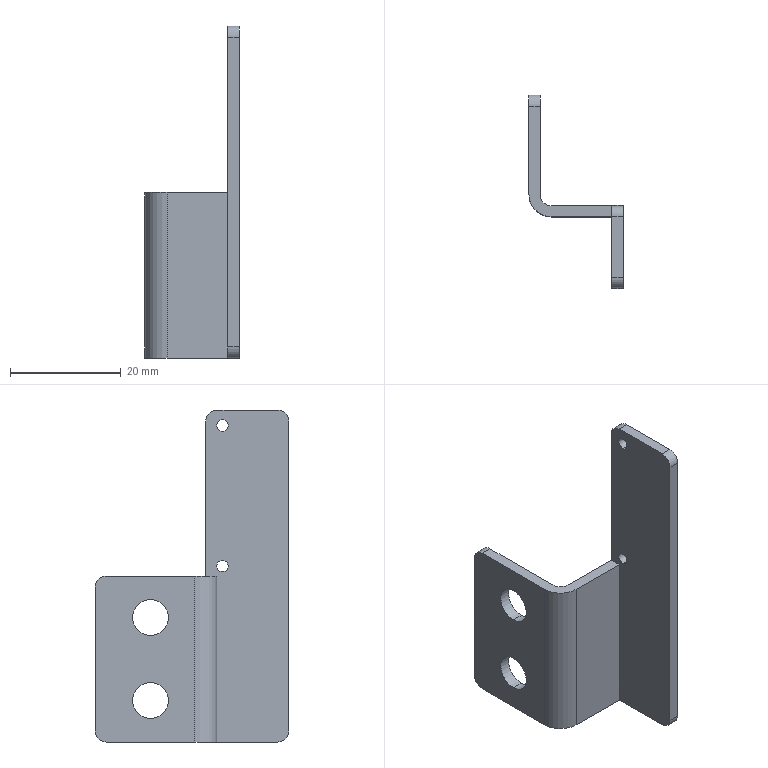Part | STEP file | 11-XDS-01-03511 | 1 solid | 26 faces | box 17 x 35 x 60 mm | volume 3668 mm3 | cylinder 15 | plane 11 | commonest cylinder face diameters 4 x6 2.05 x4 6.5 x4 8 x1
STEP:
#1=CARTESIAN_POINT('',(13.,-3.,58.225));
#2=VERTEX_POINT('',#1);
#3=CARTESIAN_POINT('',(13.,-3.,56.175));
#4=VERTEX_POINT('',#3);
#5=CARTESIAN_POINT('',(13.,-3.,57.2));
#6=DIRECTION('',(1.,0.,0.));
#7=DIRECTION('',(0.,1.,0.));
#8=AXIS2_PLACEMENT_3D('',#5,#6,#7);
#9=CIRCLE('',#8,1.025);
#10=EDGE_CURVE('',#2,#4,#9,.T.);
#11=ORIENTED_EDGE('',*,*,#10,.F.);
#12=CARTESIAN_POINT('',(15.,-3.,58.225));
#13=VERTEX_POINT('',#12);
#14=CARTESIAN_POINT('',(15.,-3.,58.225));
#15=DIRECTION('',(1.,0.,0.));
#16=VECTOR('',#15,1000.);
#17=LINE('',#14,#16);
#18=EDGE_CURVE('',#2,#13,#17,.T.);
#19=ORIENTED_EDGE('',*,*,#18,.T.);
#20=CARTESIAN_POINT('',(15.,-3.,56.175));
#21=VERTEX_POINT('',#20);
#22=CARTESIAN_POINT('',(15.,-3.,57.2));
#23=DIRECTION('',(1.,0.,0.));
#24=DIRECTION('',(0.,0.,-1.));
#25=AXIS2_PLACEMENT_3D('',#22,#23,#24);
#26=CIRCLE('',#25,1.025);
#27=EDGE_CURVE('',#13,#21,#26,.T.);
#28=ORIENTED_EDGE('',*,*,#27,.T.);
#29=CARTESIAN_POINT('',(15.,-3.,56.175));
#30=DIRECTION('',(1.,0.,0.));
#31=VECTOR('',#30,1000.);
#32=LINE('',#29,#31);
#33=EDGE_CURVE('',#4,#21,#32,.T.);
#34=ORIENTED_EDGE('',*,*,#33,.F.);
#35=EDGE_LOOP('',(#11,#19,#28,#34));
#36=FACE_OUTER_BOUND('',#35,.T.);
#37=CARTESIAN_POINT('',(15.,-3.,57.2));
#38=DIRECTION('',(1.,0.,0.));
#39=DIRECTION('',(0.,0.,-1.));
#40=AXIS2_PLACEMENT_3D('',#37,#38,#39);
#41=CYLINDRICAL_SURFACE('',#40,1.025);
#42=ADVANCED_FACE('',(#36),#41,.F.);
#43=CARTESIAN_POINT('',(13.,-3.,32.825));
#44=VERTEX_POINT('',#43);
#45=CARTESIAN_POINT('',(13.,-3.,30.775));
#46=VERTEX_POINT('',#45);
#47=CARTESIAN_POINT('',(13.,-3.,31.8));
#48=DIRECTION('',(1.,0.,0.));
#49=DIRECTION('',(0.,1.,0.));
#50=AXIS2_PLACEMENT_3D('',#47,#48,#49);
#51=CIRCLE('',#50,1.025);
#52=EDGE_CURVE('',#44,#46,#51,.T.);
#53=ORIENTED_EDGE('',*,*,#52,.F.);
#54=CARTESIAN_POINT('',(15.,-3.,32.825));
#55=VERTEX_POINT('',#54);
#56=CARTESIAN_POINT('',(15.,-3.,32.825));
#57=DIRECTION('',(1.,0.,0.));
#58=VECTOR('',#57,1000.);
#59=LINE('',#56,#58);
#60=EDGE_CURVE('',#44,#55,#59,.T.);
#61=ORIENTED_EDGE('',*,*,#60,.T.);
#62=CARTESIAN_POINT('',(15.,-3.,30.775));
#63=VERTEX_POINT('',#62);
#64=CARTESIAN_POINT('',(15.,-3.,31.8));
#65=DIRECTION('',(1.,0.,0.));
#66=DIRECTION('',(0.,0.,-1.));
#67=AXIS2_PLACEMENT_3D('',#64,#65,#66);
#68=CIRCLE('',#67,1.025);
#69=EDGE_CURVE('',#55,#63,#68,.T.);
#70=ORIENTED_EDGE('',*,*,#69,.T.);
#71=CARTESIAN_POINT('',(15.,-3.,30.775));
#72=DIRECTION('',(1.,0.,0.));
#73=VECTOR('',#72,1000.);
#74=LINE('',#71,#73);
#75=EDGE_CURVE('',#46,#63,#74,.T.);
#76=ORIENTED_EDGE('',*,*,#75,.F.);
#77=EDGE_LOOP('',(#53,#61,#70,#76));
#78=FACE_OUTER_BOUND('',#77,.T.);
#79=CARTESIAN_POINT('',(15.,-3.,31.8));
#80=DIRECTION('',(1.,0.,0.));
#81=DIRECTION('',(0.,0.,-1.));
#82=AXIS2_PLACEMENT_3D('',#79,#80,#81);
#83=CYLINDRICAL_SURFACE('',#82,1.025);
#84=ADVANCED_FACE('',(#78),#83,.F.);
#85=CARTESIAN_POINT('',(-2.,10.,10.75));
#86=VERTEX_POINT('',#85);
#87=CARTESIAN_POINT('',(-2.,10.,4.25));
#88=VERTEX_POINT('',#87);
#89=CARTESIAN_POINT('',(-2.,10.,7.5));
#90=DIRECTION('',(1.,0.,0.));
#91=DIRECTION('',(0.,0.,-1.));
#92=AXIS2_PLACEMENT_3D('',#89,#90,#91);
#93=CIRCLE('',#92,3.25);
#94=EDGE_CURVE('',#86,#88,#93,.T.);
#95=ORIENTED_EDGE('',*,*,#94,.F.);
#96=CARTESIAN_POINT('',(0.,10.,10.75));
#97=VERTEX_POINT('',#96);
#98=CARTESIAN_POINT('',(-20.,10.,10.75));
#99=DIRECTION('',(1.,0.,0.));
#100=VECTOR('',#99,1000.);
#101=LINE('',#98,#100);
#102=EDGE_CURVE('',#86,#97,#101,.T.);
#103=ORIENTED_EDGE('',*,*,#102,.T.);
#104=CARTESIAN_POINT('',(0.,10.,4.25));
#105=VERTEX_POINT('',#104);
#106=CARTESIAN_POINT('',(0.,10.,7.5));
#107=DIRECTION('',(1.,0.,0.));
#108=DIRECTION('',(0.,0.,-1.));
#109=AXIS2_PLACEMENT_3D('',#106,#107,#108);
#110=CIRCLE('',#109,3.25);
#111=EDGE_CURVE('',#97,#105,#110,.T.);
#112=ORIENTED_EDGE('',*,*,#111,.T.);
#113=CARTESIAN_POINT('',(-20.,10.,4.25));
#114=DIRECTION('',(1.,0.,0.));
#115=VECTOR('',#114,1000.);
#116=LINE('',#113,#115);
#117=EDGE_CURVE('',#88,#105,#116,.T.);
#118=ORIENTED_EDGE('',*,*,#117,.F.);
#119=EDGE_LOOP('',(#95,#103,#112,#118));
#120=FACE_OUTER_BOUND('',#119,.T.);
#121=CARTESIAN_POINT('',(-20.,10.,7.5));
#122=DIRECTION('',(1.,0.,0.));
#123=DIRECTION('',(0.,0.,-1.));
#124=AXIS2_PLACEMENT_3D('',#121,#122,#123);
#125=CYLINDRICAL_SURFACE('',#124,3.25);
#126=ADVANCED_FACE('',(#120),#125,.F.);
#127=CARTESIAN_POINT('',(-2.,10.,25.75));
#128=VERTEX_POINT('',#127);
#129=CARTESIAN_POINT('',(-2.,10.,19.25));
#130=VERTEX_POINT('',#129);
#131=CARTESIAN_POINT('',(-2.,10.,22.5));
#132=DIRECTION('',(1.,0.,0.));
#133=DIRECTION('',(0.,0.,-1.));
#134=AXIS2_PLACEMENT_3D('',#131,#132,#133);
#135=CIRCLE('',#134,3.25);
#136=EDGE_CURVE('',#128,#130,#135,.T.);
#137=ORIENTED_EDGE('',*,*,#136,.F.);
#138=CARTESIAN_POINT('',(0.,10.,25.75));
#139=VERTEX_POINT('',#138);
#140=CARTESIAN_POINT('',(-20.,10.,25.75));
#141=DIRECTION('',(1.,0.,0.));
#142=VECTOR('',#141,1000.);
#143=LINE('',#140,#142);
#144=EDGE_CURVE('',#128,#139,#143,.T.);
#145=ORIENTED_EDGE('',*,*,#144,.T.);
#146=CARTESIAN_POINT('',(0.,10.,19.25));
#147=VERTEX_POINT('',#146);
#148=CARTESIAN_POINT('',(0.,10.,22.5));
#149=DIRECTION('',(1.,0.,0.));
#150=DIRECTION('',(0.,0.,-1.));
#151=AXIS2_PLACEMENT_3D('',#148,#149,#150);
#152=CIRCLE('',#151,3.25);
#153=EDGE_CURVE('',#139,#147,#152,.T.);
#154=ORIENTED_EDGE('',*,*,#153,.T.);
#155=CARTESIAN_POINT('',(-20.,10.,19.25));
#156=DIRECTION('',(1.,0.,0.));
#157=VECTOR('',#156,1000.);
#158=LINE('',#155,#157);
#159=EDGE_CURVE('',#130,#147,#158,.T.);
#160=ORIENTED_EDGE('',*,*,#159,.F.);
#161=EDGE_LOOP('',(#137,#145,#154,#160));
#162=FACE_OUTER_BOUND('',#161,.T.);
#163=CARTESIAN_POINT('',(-20.,10.,22.5));
#164=DIRECTION('',(1.,0.,0.));
#165=DIRECTION('',(0.,0.,-1.));
#166=AXIS2_PLACEMENT_3D('',#163,#164,#165);
#167=CYLINDRICAL_SURFACE('',#166,3.25);
#168=ADVANCED_FACE('',(#162),#167,.F.);
#169=CARTESIAN_POINT('',(13.,-3.,57.2));
#170=DIRECTION('',(1.,0.,0.));
#171=DIRECTION('',(0.,1.,0.));
#172=AXIS2_PLACEMENT_3D('',#169,#170,#171);
#173=CIRCLE('',#172,1.025);
#174=EDGE_CURVE('',#4,#2,#173,.T.);
#175=ORIENTED_EDGE('',*,*,#174,.T.);
#176=ORIENTED_EDGE('',*,*,#10,.T.);
#177=EDGE_LOOP('',(#175,#176));
#178=FACE_BOUND('',#177,.T.);
#179=CARTESIAN_POINT('',(13.,-3.,31.8));
#180=DIRECTION('',(1.,0.,0.));
#181=DIRECTION('',(0.,1.,0.));
#182=AXIS2_PLACEMENT_3D('',#179,#180,#181);
#183=CIRCLE('',#182,1.025);
#184=EDGE_CURVE('',#46,#44,#183,.T.);
#185=ORIENTED_EDGE('',*,*,#184,.T.);
#186=ORIENTED_EDGE('',*,*,#52,.T.);
#187=EDGE_LOOP('',(#185,#186));
#188=FACE_BOUND('',#187,.T.);
#189=CARTESIAN_POINT('',(13.,-2.,0.));
#190=VERTEX_POINT('',#189);
#191=CARTESIAN_POINT('',(13.,-13.,0.));
#192=VERTEX_POINT('',#191);
#193=CARTESIAN_POINT('',(13.,0.,0.));
#194=DIRECTION('',(0.,-1.,0.));
#195=VECTOR('',#194,1000.);
#196=LINE('',#193,#195);
#197=EDGE_CURVE('',#190,#192,#196,.T.);
#198=ORIENTED_EDGE('',*,*,#197,.T.);
#199=CARTESIAN_POINT('',(13.,-15.,2.));
#200=VERTEX_POINT('',#199);
#201=CARTESIAN_POINT('',(13.,-13.,2.));
#202=DIRECTION('',(-1.,0.,0.));
#203=DIRECTION('',(0.,1.,0.));
#204=AXIS2_PLACEMENT_3D('',#201,#202,#203);
#205=CIRCLE('',#204,2.);
#206=EDGE_CURVE('',#192,#200,#205,.T.);
#207=ORIENTED_EDGE('',*,*,#206,.T.);
#208=CARTESIAN_POINT('',(13.,-15.,58.));
#209=VERTEX_POINT('',#208);
#210=CARTESIAN_POINT('',(13.,-15.,30.));
#211=DIRECTION('',(0.,0.,-1.));
#212=VECTOR('',#211,1000.);
#213=LINE('',#210,#212);
#214=EDGE_CURVE('',#209,#200,#213,.T.);
#215=ORIENTED_EDGE('',*,*,#214,.F.);
#216=CARTESIAN_POINT('',(13.,-13.,60.));
#217=VERTEX_POINT('',#216);
#218=CARTESIAN_POINT('',(13.,-13.,58.));
#219=DIRECTION('',(-1.,0.,0.));
#220=DIRECTION('',(0.,1.,0.));
#221=AXIS2_PLACEMENT_3D('',#218,#219,#220);
#222=CIRCLE('',#221,2.);
#223=EDGE_CURVE('',#209,#217,#222,.T.);
#224=ORIENTED_EDGE('',*,*,#223,.T.);
#225=CARTESIAN_POINT('',(13.,-2.,60.));
#226=VERTEX_POINT('',#225);
#227=CARTESIAN_POINT('',(13.,-15.,60.));
#228=DIRECTION('',(0.,-1.,0.));
#229=VECTOR('',#228,1000.);
#230=LINE('',#227,#229);
#231=EDGE_CURVE('',#226,#217,#230,.T.);
#232=ORIENTED_EDGE('',*,*,#231,.F.);
#233=CARTESIAN_POINT('',(13.,0.,58.));
#234=VERTEX_POINT('',#233);
#235=CARTESIAN_POINT('',(13.,-2.,58.));
#236=DIRECTION('',(-1.,0.,0.));
#237=DIRECTION('',(0.,1.,0.));
#238=AXIS2_PLACEMENT_3D('',#235,#236,#237);
#239=CIRCLE('',#238,2.);
#240=EDGE_CURVE('',#226,#234,#239,.T.);
#241=ORIENTED_EDGE('',*,*,#240,.T.);
#242=CARTESIAN_POINT('',(13.,0.,30.));
#243=VERTEX_POINT('',#242);
#244=CARTESIAN_POINT('',(13.,0.,60.));
#245=DIRECTION('',(0.,0.,-1.));
#246=VECTOR('',#245,1000.);
#247=LINE('',#244,#246);
#248=EDGE_CURVE('',#234,#243,#247,.T.);
#249=ORIENTED_EDGE('',*,*,#248,.T.);
#250=CARTESIAN_POINT('',(13.,-2.,30.));
#251=VERTEX_POINT('',#250);
#252=CARTESIAN_POINT('',(13.,-15.,30.));
#253=DIRECTION('',(0.,-1.,0.));
#254=VECTOR('',#253,1000.);
#255=LINE('',#252,#254);
#256=EDGE_CURVE('',#243,#251,#255,.T.);
#257=ORIENTED_EDGE('',*,*,#256,.T.);
#258=CARTESIAN_POINT('',(13.,-2.,30.));
#259=DIRECTION('',(0.,0.,-1.));
#260=VECTOR('',#259,1000.);
#261=LINE('',#258,#260);
#262=EDGE_CURVE('',#251,#190,#261,.T.);
#263=ORIENTED_EDGE('',*,*,#262,.T.);
#264=EDGE_LOOP('',(#198,#207,#215,#224,#232,#241,#249,#257,#263));
#265=FACE_OUTER_BOUND('',#264,.T.);
#266=CARTESIAN_POINT('',(13.,0.,30.));
#267=DIRECTION('',(1.,0.,0.));
#268=DIRECTION('',(0.,1.,0.));
#269=AXIS2_PLACEMENT_3D('',#266,#267,#268);
#270=PLANE('',#269);
#271=ADVANCED_FACE('',(#178,#188,#265),#270,.F.);
#272=ORIENTED_EDGE('',*,*,#214,.T.);
#273=CARTESIAN_POINT('',(15.,-15.,2.));
#274=VERTEX_POINT('',#273);
#275=CARTESIAN_POINT('',(15.,-15.,2.));
#276=DIRECTION('',(1.,0.,0.));
#277=VECTOR('',#276,1000.);
#278=LINE('',#275,#277);
#279=EDGE_CURVE('',#200,#274,#278,.T.);
#280=ORIENTED_EDGE('',*,*,#279,.T.);
#281=CARTESIAN_POINT('',(15.,-15.,58.));
#282=VERTEX_POINT('',#281);
#283=CARTESIAN_POINT('',(15.,-15.,30.));
#284=DIRECTION('',(0.,0.,-1.));
#285=VECTOR('',#284,1000.);
#286=LINE('',#283,#285);
#287=EDGE_CURVE('',#282,#274,#286,.T.);
#288=ORIENTED_EDGE('',*,*,#287,.F.);
#289=CARTESIAN_POINT('',(13.,-15.,58.));
#290=DIRECTION('',(-1.,0.,0.));
#291=VECTOR('',#290,1000.);
#292=LINE('',#289,#291);
#293=EDGE_CURVE('',#282,#209,#292,.T.);
#294=ORIENTED_EDGE('',*,*,#293,.T.);
#295=EDGE_LOOP('',(#272,#280,#288,#294));
#296=FACE_OUTER_BOUND('',#295,.T.);
#297=CARTESIAN_POINT('',(15.,-15.,30.));
#298=DIRECTION('',(0.,-1.,0.));
#299=DIRECTION('',(0.,0.,-1.));
#300=AXIS2_PLACEMENT_3D('',#297,#298,#299);
#301=PLANE('',#300);
#302=ADVANCED_FACE('',(#296),#301,.T.);
#303=CARTESIAN_POINT('',(15.,-3.,57.2));
#304=DIRECTION('',(1.,0.,0.));
#305=DIRECTION('',(0.,0.,-1.));
#306=AXIS2_PLACEMENT_3D('',#303,#304,#305);
#307=CIRCLE('',#306,1.025);
#308=EDGE_CURVE('',#21,#13,#307,.T.);
#309=ORIENTED_EDGE('',*,*,#308,.F.);
#310=ORIENTED_EDGE('',*,*,#27,.F.);
#311=EDGE_LOOP('',(#309,#310));
#312=FACE_BOUND('',#311,.T.);
#313=CARTESIAN_POINT('',(15.,-3.,31.8));
#314=DIRECTION('',(1.,0.,0.));
#315=DIRECTION('',(0.,0.,-1.));
#316=AXIS2_PLACEMENT_3D('',#313,#314,#315);
#317=CIRCLE('',#316,1.025);
#318=EDGE_CURVE('',#63,#55,#317,.T.);
#319=ORIENTED_EDGE('',*,*,#318,.F.);
#320=ORIENTED_EDGE('',*,*,#69,.F.);
#321=EDGE_LOOP('',(#319,#320));
#322=FACE_BOUND('',#321,.T.);
#323=ORIENTED_EDGE('',*,*,#287,.T.);
#324=CARTESIAN_POINT('',(15.,-13.,0.));
#325=VERTEX_POINT('',#324);
#326=CARTESIAN_POINT('',(15.,-13.,2.));
#327=DIRECTION('',(1.,0.,0.));
#328=DIRECTION('',(0.,1.,0.));
#329=AXIS2_PLACEMENT_3D('',#326,#327,#328);
#330=CIRCLE('',#329,2.);
#331=EDGE_CURVE('',#274,#325,#330,.T.);
#332=ORIENTED_EDGE('',*,*,#331,.T.);
#333=CARTESIAN_POINT('',(15.,0.,0.));
#334=VERTEX_POINT('',#333);
#335=CARTESIAN_POINT('',(15.,0.,0.));
#336=DIRECTION('',(0.,-1.,0.));
#337=VECTOR('',#336,1000.);
#338=LINE('',#335,#337);
#339=EDGE_CURVE('',#334,#325,#338,.T.);
#340=ORIENTED_EDGE('',*,*,#339,.F.);
#341=CARTESIAN_POINT('',(15.,0.,58.));
#342=VERTEX_POINT('',#341);
#343=CARTESIAN_POINT('',(15.,0.,30.));
#344=DIRECTION('',(0.,0.,-1.));
#345=VECTOR('',#344,1000.);
#346=LINE('',#343,#345);
#347=EDGE_CURVE('',#342,#334,#346,.T.);
#348=ORIENTED_EDGE('',*,*,#347,.F.);
#349=CARTESIAN_POINT('',(15.,-2.,60.));
#350=VERTEX_POINT('',#349);
#351=CARTESIAN_POINT('',(15.,-2.,58.));
#352=DIRECTION('',(1.,0.,0.));
#353=DIRECTION('',(0.,1.,0.));
#354=AXIS2_PLACEMENT_3D('',#351,#352,#353);
#355=CIRCLE('',#354,2.);
#356=EDGE_CURVE('',#342,#350,#355,.T.);
#357=ORIENTED_EDGE('',*,*,#356,.T.);
#358=CARTESIAN_POINT('',(15.,-13.,60.));
#359=VERTEX_POINT('',#358);
#360=CARTESIAN_POINT('',(15.,-15.,60.));
#361=DIRECTION('',(0.,1.,0.));
#362=VECTOR('',#361,1000.);
#363=LINE('',#360,#362);
#364=EDGE_CURVE('',#359,#350,#363,.T.);
#365=ORIENTED_EDGE('',*,*,#364,.F.);
#366=CARTESIAN_POINT('',(15.,-13.,58.));
#367=DIRECTION('',(1.,0.,0.));
#368=DIRECTION('',(0.,1.,0.));
#369=AXIS2_PLACEMENT_3D('',#366,#367,#368);
#370=CIRCLE('',#369,2.);
#371=EDGE_CURVE('',#359,#282,#370,.T.);
#372=ORIENTED_EDGE('',*,*,#371,.T.);
#373=EDGE_LOOP('',(#323,#332,#340,#348,#357,#365,#372));
#374=FACE_OUTER_BOUND('',#373,.T.);
#375=CARTESIAN_POINT('',(15.,0.,30.));
#376=DIRECTION('',(1.,0.,0.));
#377=DIRECTION('',(0.,1.,0.));
#378=AXIS2_PLACEMENT_3D('',#375,#376,#377);
#379=PLANE('',#378);
#380=ADVANCED_FACE('',(#312,#322,#374),#379,.T.);
#381=ORIENTED_EDGE('',*,*,#248,.F.);
#382=CARTESIAN_POINT('',(15.,0.,58.));
#383=DIRECTION('',(1.,0.,0.));
#384=VECTOR('',#383,1000.);
#385=LINE('',#382,#384);
#386=EDGE_CURVE('',#234,#342,#385,.T.);
#387=ORIENTED_EDGE('',*,*,#386,.T.);
#388=ORIENTED_EDGE('',*,*,#347,.T.);
#389=CARTESIAN_POINT('',(2.,0.,0.));
#390=VERTEX_POINT('',#389);
#391=CARTESIAN_POINT('',(2.,0.,0.));
#392=DIRECTION('',(1.,0.,0.));
#393=VECTOR('',#392,1000.);
#394=LINE('',#391,#393);
#395=EDGE_CURVE('',#390,#334,#394,.T.);
#396=ORIENTED_EDGE('',*,*,#395,.F.);
#397=CARTESIAN_POINT('',(2.,0.,30.));
#398=VERTEX_POINT('',#397);
#399=CARTESIAN_POINT('',(2.,0.,30.));
#400=DIRECTION('',(0.,0.,-1.));
#401=VECTOR('',#400,1000.);
#402=LINE('',#399,#401);
#403=EDGE_CURVE('',#398,#390,#402,.T.);
#404=ORIENTED_EDGE('',*,*,#403,.F.);
#405=CARTESIAN_POINT('',(2.,0.,30.));
#406=DIRECTION('',(1.,0.,0.));
#407=VECTOR('',#406,1000.);
#408=LINE('',#405,#407);
#409=EDGE_CURVE('',#398,#243,#408,.T.);
#410=ORIENTED_EDGE('',*,*,#409,.T.);
#411=EDGE_LOOP('',(#381,#387,#388,#396,#404,#410));
#412=FACE_OUTER_BOUND('',#411,.T.);
#413=CARTESIAN_POINT('',(2.,0.,30.));
#414=DIRECTION('',(0.,1.,0.));
#415=DIRECTION('',(0.,0.,1.));
#416=AXIS2_PLACEMENT_3D('',#413,#414,#415);
#417=PLANE('',#416);
#418=ADVANCED_FACE('',(#412),#417,.T.);
#419=CARTESIAN_POINT('',(0.,2.,0.));
#420=VERTEX_POINT('',#419);
#421=CARTESIAN_POINT('',(2.,2.,0.));
#422=DIRECTION('',(0.,0.,1.));
#423=DIRECTION('',(1.,0.,0.));
#424=AXIS2_PLACEMENT_3D('',#421,#422,#423);
#425=CIRCLE('',#424,2.);
#426=EDGE_CURVE('',#420,#390,#425,.T.);
#427=ORIENTED_EDGE('',*,*,#426,.F.);
#428=CARTESIAN_POINT('',(0.,2.,30.));
#429=VERTEX_POINT('',#428);
#430=CARTESIAN_POINT('',(0.,2.,30.));
#431=DIRECTION('',(0.,0.,-1.));
#432=VECTOR('',#431,1000.);
#433=LINE('',#430,#432);
#434=EDGE_CURVE('',#429,#420,#433,.T.);
#435=ORIENTED_EDGE('',*,*,#434,.F.);
#436=CARTESIAN_POINT('',(2.,2.,30.));
#437=DIRECTION('',(0.,0.,1.));
#438=DIRECTION('',(1.,0.,0.));
#439=AXIS2_PLACEMENT_3D('',#436,#437,#438);
#440=CIRCLE('',#439,2.);
#441=EDGE_CURVE('',#429,#398,#440,.T.);
#442=ORIENTED_EDGE('',*,*,#441,.T.);
#443=ORIENTED_EDGE('',*,*,#403,.T.);
#444=EDGE_LOOP('',(#427,#435,#442,#443));
#445=FACE_OUTER_BOUND('',#444,.T.);
#446=CARTESIAN_POINT('',(2.,2.,30.));
#447=DIRECTION('',(0.,0.,-1.));
#448=DIRECTION('',(-1.,0.,0.));
#449=AXIS2_PLACEMENT_3D('',#446,#447,#448);
#450=CYLINDRICAL_SURFACE('',#449,2.);
#451=ADVANCED_FACE('',(#445),#450,.F.);
#452=CARTESIAN_POINT('',(0.,10.,7.5));
#453=DIRECTION('',(1.,0.,0.));
#454=DIRECTION('',(0.,0.,-1.));
#455=AXIS2_PLACEMENT_3D('',#452,#453,#454);
#456=CIRCLE('',#455,3.25);
#457=EDGE_CURVE('',#105,#97,#456,.T.);
#458=ORIENTED_EDGE('',*,*,#457,.F.);
#459=ORIENTED_EDGE('',*,*,#111,.F.);
#460=EDGE_LOOP('',(#458,#459));
#461=FACE_BOUND('',#460,.T.);
#462=CARTESIAN_POINT('',(0.,10.,22.5));
#463=DIRECTION('',(1.,0.,0.));
#464=DIRECTION('',(0.,0.,-1.));
#465=AXIS2_PLACEMENT_3D('',#462,#463,#464);
#466=CIRCLE('',#465,3.25);
#467=EDGE_CURVE('',#147,#139,#466,.T.);
#468=ORIENTED_EDGE('',*,*,#467,.F.);
#469=ORIENTED_EDGE('',*,*,#153,.F.);
#470=EDGE_LOOP('',(#468,#469));
#471=FACE_BOUND('',#470,.T.);
#472=CARTESIAN_POINT('',(0.,18.,0.));
#473=VERTEX_POINT('',#472);
#474=CARTESIAN_POINT('',(0.,20.,0.));
#475=DIRECTION('',(0.,-1.,0.));
#476=VECTOR('',#475,1000.);
#477=LINE('',#474,#476);
#478=EDGE_CURVE('',#473,#420,#477,.T.);
#479=ORIENTED_EDGE('',*,*,#478,.F.);
#480=CARTESIAN_POINT('',(0.,20.,2.));
#481=VERTEX_POINT('',#480);
#482=CARTESIAN_POINT('',(0.,18.,2.));
#483=DIRECTION('',(1.,0.,0.));
#484=DIRECTION('',(0.,0.,-1.));
#485=AXIS2_PLACEMENT_3D('',#482,#483,#484);
#486=CIRCLE('',#485,2.);
#487=EDGE_CURVE('',#473,#481,#486,.T.);
#488=ORIENTED_EDGE('',*,*,#487,.T.);
#489=CARTESIAN_POINT('',(0.,20.,28.));
#490=VERTEX_POINT('',#489);
#491=CARTESIAN_POINT('',(0.,20.,30.));
#492=DIRECTION('',(0.,0.,-1.));
#493=VECTOR('',#492,1000.);
#494=LINE('',#491,#493);
#495=EDGE_CURVE('',#490,#481,#494,.T.);
#496=ORIENTED_EDGE('',*,*,#495,.F.);
#497=CARTESIAN_POINT('',(0.,18.,30.));
#498=VERTEX_POINT('',#497);
#499=CARTESIAN_POINT('',(0.,18.,28.));
#500=DIRECTION('',(1.,0.,0.));
#501=DIRECTION('',(0.,0.,-1.));
#502=AXIS2_PLACEMENT_3D('',#499,#500,#501);
#503=CIRCLE('',#502,2.);
#504=EDGE_CURVE('',#490,#498,#503,.T.);
#505=ORIENTED_EDGE('',*,*,#504,.T.);
#506=CARTESIAN_POINT('',(0.,20.,30.));
#507=DIRECTION('',(0.,-1.,0.));
#508=VECTOR('',#507,1000.);
#509=LINE('',#506,#508);
#510=EDGE_CURVE('',#498,#429,#509,.T.);
#511=ORIENTED_EDGE('',*,*,#510,.T.);
#512=ORIENTED_EDGE('',*,*,#434,.T.);
#513=EDGE_LOOP('',(#479,#488,#496,#505,#511,#512));
#514=FACE_OUTER_BOUND('',#513,.T.);
#515=CARTESIAN_POINT('',(0.,20.,30.));
#516=DIRECTION('',(1.,0.,0.));
#517=DIRECTION('',(0.,0.,-1.));
#518=AXIS2_PLACEMENT_3D('',#515,#516,#517);
#519=PLANE('',#518);
#520=ADVANCED_FACE('',(#461,#471,#514),#519,.T.);
#521=ORIENTED_EDGE('',*,*,#495,.T.);
#522=CARTESIAN_POINT('',(-2.,20.,2.));
#523=VERTEX_POINT('',#522);
#524=CARTESIAN_POINT('',(-2.,20.,2.));
#525=DIRECTION('',(-1.,0.,0.));
#526=VECTOR('',#525,1000.);
#527=LINE('',#524,#526);
#528=EDGE_CURVE('',#481,#523,#527,.T.);
#529=ORIENTED_EDGE('',*,*,#528,.T.);
#530=CARTESIAN_POINT('',(-2.,20.,28.));
#531=VERTEX_POINT('',#530);
#532=CARTESIAN_POINT('',(-2.,20.,30.));
#533=DIRECTION('',(0.,0.,-1.));
#534=VECTOR('',#533,1000.);
#535=LINE('',#532,#534);
#536=EDGE_CURVE('',#531,#523,#535,.T.);
#537=ORIENTED_EDGE('',*,*,#536,.F.);
#538=CARTESIAN_POINT('',(-2.,20.,28.));
#539=DIRECTION('',(1.,0.,0.));
#540=VECTOR('',#539,1000.);
#541=LINE('',#538,#540);
#542=EDGE_CURVE('',#531,#490,#541,.T.);
#543=ORIENTED_EDGE('',*,*,#542,.T.);
#544=EDGE_LOOP('',(#521,#529,#537,#543));
#545=FACE_OUTER_BOUND('',#544,.T.);
#546=CARTESIAN_POINT('',(-2.,20.,30.));
#547=DIRECTION('',(0.,1.,0.));
#548=DIRECTION('',(0.,0.,1.));
#549=AXIS2_PLACEMENT_3D('',#546,#547,#548);
#550=PLANE('',#549);
#551=ADVANCED_FACE('',(#545),#550,.T.);
#552=CARTESIAN_POINT('',(-2.,10.,7.5));
#553=DIRECTION('',(1.,0.,0.));
#554=DIRECTION('',(0.,0.,-1.));
#555=AXIS2_PLACEMENT_3D('',#552,#553,#554);
#556=CIRCLE('',#555,3.25);
#557=EDGE_CURVE('',#88,#86,#556,.T.);
#558=ORIENTED_EDGE('',*,*,#557,.T.);
#559=ORIENTED_EDGE('',*,*,#94,.T.);
#560=EDGE_LOOP('',(#558,#559));
#561=FACE_BOUND('',#560,.T.);
#562=CARTESIAN_POINT('',(-2.,10.,22.5));
#563=DIRECTION('',(1.,0.,0.));
#564=DIRECTION('',(0.,0.,-1.));
#565=AXIS2_PLACEMENT_3D('',#562,#563,#564);
#566=CIRCLE('',#565,3.25);
#567=EDGE_CURVE('',#130,#128,#566,.T.);
#568=ORIENTED_EDGE('',*,*,#567,.T.);
#569=ORIENTED_EDGE('',*,*,#136,.T.);
#570=EDGE_LOOP('',(#568,#569));
#571=FACE_BOUND('',#570,.T.);
#572=ORIENTED_EDGE('',*,*,#536,.T.);
#573=CARTESIAN_POINT('',(-2.,18.,0.));
#574=VERTEX_POINT('',#573);
#575=CARTESIAN_POINT('',(-2.,18.,2.));
#576=DIRECTION('',(-1.,0.,0.));
#577=DIRECTION('',(0.,0.,-1.));
#578=AXIS2_PLACEMENT_3D('',#575,#576,#577);
#579=CIRCLE('',#578,2.);
#580=EDGE_CURVE('',#523,#574,#579,.T.);
#581=ORIENTED_EDGE('',*,*,#580,.T.);
#582=CARTESIAN_POINT('',(-2.,2.,0.));
#583=VERTEX_POINT('',#582);
#584=CARTESIAN_POINT('',(-2.,20.,0.));
#585=DIRECTION('',(0.,-1.,0.));
#586=VECTOR('',#585,1000.);
#587=LINE('',#584,#586);
#588=EDGE_CURVE('',#574,#583,#587,.T.);
#589=ORIENTED_EDGE('',*,*,#588,.T.);
#590=CARTESIAN_POINT('',(-2.,2.,30.));
#591=VERTEX_POINT('',#590);
#592=CARTESIAN_POINT('',(-2.,2.,30.));
#593=DIRECTION('',(0.,0.,-1.));
#594=VECTOR('',#593,1000.);
#595=LINE('',#592,#594);
#596=EDGE_CURVE('',#591,#583,#595,.T.);
#597=ORIENTED_EDGE('',*,*,#596,.F.);
#598=CARTESIAN_POINT('',(-2.,18.,30.));
#599=VERTEX_POINT('',#598);
#600=CARTESIAN_POINT('',(-2.,20.,30.));
#601=DIRECTION('',(0.,-1.,0.));
#602=VECTOR('',#601,1000.);
#603=LINE('',#600,#602);
#604=EDGE_CURVE('',#599,#591,#603,.T.);
#605=ORIENTED_EDGE('',*,*,#604,.F.);
#606=CARTESIAN_POINT('',(-2.,18.,28.));
#607=DIRECTION('',(-1.,0.,0.));
#608=DIRECTION('',(0.,0.,-1.));
#609=AXIS2_PLACEMENT_3D('',#606,#607,#608);
#610=CIRCLE('',#609,2.);
#611=EDGE_CURVE('',#599,#531,#610,.T.);
#612=ORIENTED_EDGE('',*,*,#611,.T.);
#613=EDGE_LOOP('',(#572,#581,#589,#597,#605,#612));
#614=FACE_OUTER_BOUND('',#613,.T.);
#615=CARTESIAN_POINT('',(-2.,20.,30.));
#616=DIRECTION('',(1.,0.,0.));
#617=DIRECTION('',(0.,0.,-1.));
#618=AXIS2_PLACEMENT_3D('',#615,#616,#617);
#619=PLANE('',#618);
#620=ADVANCED_FACE('',(#561,#571,#614),#619,.F.);
#621=CARTESIAN_POINT('',(2.,-2.,0.));
#622=VERTEX_POINT('',#621);
#623=CARTESIAN_POINT('',(2.,2.,0.));
#624=DIRECTION('',(0.,0.,1.));
#625=DIRECTION('',(1.,0.,0.));
#626=AXIS2_PLACEMENT_3D('',#623,#624,#625);
#627=CIRCLE('',#626,4.);
#628=EDGE_CURVE('',#583,#622,#627,.T.);
#629=ORIENTED_EDGE('',*,*,#628,.T.);
#630=CARTESIAN_POINT('',(2.,-2.,30.));
#631=VERTEX_POINT('',#630);
#632=CARTESIAN_POINT('',(2.,-2.,30.));
#633=DIRECTION('',(0.,0.,-1.));
#634=VECTOR('',#633,1000.);
#635=LINE('',#632,#634);
#636=EDGE_CURVE('',#631,#622,#635,.T.);
#637=ORIENTED_EDGE('',*,*,#636,.F.);
#638=CARTESIAN_POINT('',(2.,2.,30.));
#639=DIRECTION('',(0.,0.,1.));
#640=DIRECTION('',(1.,0.,0.));
#641=AXIS2_PLACEMENT_3D('',#638,#639,#640);
#642=CIRCLE('',#641,4.);
#643=EDGE_CURVE('',#591,#631,#642,.T.);
#644=ORIENTED_EDGE('',*,*,#643,.F.);
#645=ORIENTED_EDGE('',*,*,#596,.T.);
#646=EDGE_LOOP('',(#629,#637,#644,#645));
#647=FACE_OUTER_BOUND('',#646,.T.);
#648=CARTESIAN_POINT('',(2.,2.,30.));
#649=DIRECTION('',(0.,0.,-1.));
#650=DIRECTION('',(-1.,0.,0.));
#651=AXIS2_PLACEMENT_3D('',#648,#649,#650);
#652=CYLINDRICAL_SURFACE('',#651,4.);
#653=ADVANCED_FACE('',(#647),#652,.T.);
#654=CARTESIAN_POINT('',(2.,-2.,0.));
#655=DIRECTION('',(1.,0.,0.));
#656=VECTOR('',#655,1000.);
#657=LINE('',#654,#656);
#658=EDGE_CURVE('',#622,#190,#657,.T.);
#659=ORIENTED_EDGE('',*,*,#658,.T.);
#660=ORIENTED_EDGE('',*,*,#262,.F.);
#661=CARTESIAN_POINT('',(2.,-2.,30.));
#662=DIRECTION('',(1.,0.,0.));
#663=VECTOR('',#662,1000.);
#664=LINE('',#661,#663);
#665=EDGE_CURVE('',#631,#251,#664,.T.);
#666=ORIENTED_EDGE('',*,*,#665,.F.);
#667=ORIENTED_EDGE('',*,*,#636,.T.);
#668=EDGE_LOOP('',(#659,#660,#666,#667));
#669=FACE_OUTER_BOUND('',#668,.T.);
#670=CARTESIAN_POINT('',(2.,-2.,30.));
#671=DIRECTION('',(0.,1.,0.));
#672=DIRECTION('',(0.,0.,1.));
#673=AXIS2_PLACEMENT_3D('',#670,#671,#672);
#674=PLANE('',#673);
#675=ADVANCED_FACE('',(#669),#674,.F.);
#676=ORIENTED_EDGE('',*,*,#510,.F.);
#677=CARTESIAN_POINT('',(2.,18.,30.));
#678=DIRECTION('',(-1.,0.,0.));
#679=VECTOR('',#678,1000.);
#680=LINE('',#677,#679);
#681=EDGE_CURVE('',#498,#599,#680,.T.);
#682=ORIENTED_EDGE('',*,*,#681,.T.);
#683=ORIENTED_EDGE('',*,*,#604,.T.);
#684=ORIENTED_EDGE('',*,*,#643,.T.);
#685=ORIENTED_EDGE('',*,*,#665,.T.);
#686=ORIENTED_EDGE('',*,*,#256,.F.);
#687=ORIENTED_EDGE('',*,*,#409,.F.);
#688=ORIENTED_EDGE('',*,*,#441,.F.);
#689=EDGE_LOOP('',(#676,#682,#683,#684,#685,#686,#687,#688));
#690=FACE_OUTER_BOUND('',#689,.T.);
#691=CARTESIAN_POINT('',(2.,2.,30.));
#692=DIRECTION('',(0.,0.,1.));
#693=DIRECTION('',(1.,0.,0.));
#694=AXIS2_PLACEMENT_3D('',#691,#692,#693);
#695=PLANE('',#694);
#696=ADVANCED_FACE('',(#690),#695,.T.);
#697=ORIENTED_EDGE('',*,*,#339,.T.);
#698=CARTESIAN_POINT('',(13.,-13.,0.));
#699=DIRECTION('',(-1.,0.,0.));
#700=VECTOR('',#699,1000.);
#701=LINE('',#698,#700);
#702=EDGE_CURVE('',#325,#192,#701,.T.);
#703=ORIENTED_EDGE('',*,*,#702,.T.);
#704=ORIENTED_EDGE('',*,*,#197,.F.);
#705=ORIENTED_EDGE('',*,*,#658,.F.);
#706=ORIENTED_EDGE('',*,*,#628,.F.);
#707=ORIENTED_EDGE('',*,*,#588,.F.);
#708=CARTESIAN_POINT('',(0.,18.,0.));
#709=DIRECTION('',(1.,0.,0.));
#710=VECTOR('',#709,1000.);
#711=LINE('',#708,#710);
#712=EDGE_CURVE('',#574,#473,#711,.T.);
#713=ORIENTED_EDGE('',*,*,#712,.T.);
#714=ORIENTED_EDGE('',*,*,#478,.T.);
#715=ORIENTED_EDGE('',*,*,#426,.T.);
#716=ORIENTED_EDGE('',*,*,#395,.T.);
#717=EDGE_LOOP('',(#697,#703,#704,#705,#706,#707,#713,#714,#715,#716));
#718=FACE_OUTER_BOUND('',#717,.T.);
#719=CARTESIAN_POINT('',(2.,2.,0.));
#720=DIRECTION('',(0.,0.,1.));
#721=DIRECTION('',(1.,0.,0.));
#722=AXIS2_PLACEMENT_3D('',#719,#720,#721);
#723=PLANE('',#722);
#724=ADVANCED_FACE('',(#718),#723,.F.);
#725=ORIENTED_EDGE('',*,*,#231,.T.);
#726=CARTESIAN_POINT('',(15.,-13.,60.));
#727=DIRECTION('',(1.,0.,0.));
#728=VECTOR('',#727,1000.);
#729=LINE('',#726,#728);
#730=EDGE_CURVE('',#217,#359,#729,.T.);
#731=ORIENTED_EDGE('',*,*,#730,.T.);
#732=ORIENTED_EDGE('',*,*,#364,.T.);
#733=CARTESIAN_POINT('',(13.,-2.,60.));
#734=DIRECTION('',(-1.,0.,0.));
#735=VECTOR('',#734,1000.);
#736=LINE('',#733,#735);
#737=EDGE_CURVE('',#350,#226,#736,.T.);
#738=ORIENTED_EDGE('',*,*,#737,.T.);
#739=EDGE_LOOP('',(#725,#731,#732,#738));
#740=FACE_OUTER_BOUND('',#739,.T.);
#741=CARTESIAN_POINT('',(0.,0.,60.));
#742=DIRECTION('',(0.,0.,-1.));
#743=DIRECTION('',(-1.,0.,0.));
#744=AXIS2_PLACEMENT_3D('',#741,#742,#743);
#745=PLANE('',#744);
#746=ADVANCED_FACE('',(#740),#745,.F.);
#747=ORIENTED_EDGE('',*,*,#331,.F.);
#748=ORIENTED_EDGE('',*,*,#279,.F.);
#749=ORIENTED_EDGE('',*,*,#206,.F.);
#750=ORIENTED_EDGE('',*,*,#702,.F.);
#751=EDGE_LOOP('',(#747,#748,#749,#750));
#752=FACE_OUTER_BOUND('',#751,.T.);
#753=CARTESIAN_POINT('',(2.,-13.,2.));
#754=DIRECTION('',(1.,0.,0.));
#755=DIRECTION('',(0.,0.,-1.));
#756=AXIS2_PLACEMENT_3D('',#753,#754,#755);
#757=CYLINDRICAL_SURFACE('',#756,2.);
#758=ADVANCED_FACE('',(#752),#757,.T.);
#759=ORIENTED_EDGE('',*,*,#580,.F.);
#760=ORIENTED_EDGE('',*,*,#528,.F.);
#761=ORIENTED_EDGE('',*,*,#487,.F.);
#762=ORIENTED_EDGE('',*,*,#712,.F.);
#763=EDGE_LOOP('',(#759,#760,#761,#762));
#764=FACE_OUTER_BOUND('',#763,.T.);
#765=CARTESIAN_POINT('',(2.,18.,2.));
#766=DIRECTION('',(-1.,0.,0.));
#767=DIRECTION('',(0.,0.,1.));
#768=AXIS2_PLACEMENT_3D('',#765,#766,#767);
#769=CYLINDRICAL_SURFACE('',#768,2.);
#770=ADVANCED_FACE('',(#764),#769,.T.);
#771=ORIENTED_EDGE('',*,*,#611,.F.);
#772=ORIENTED_EDGE('',*,*,#681,.F.);
#773=ORIENTED_EDGE('',*,*,#504,.F.);
#774=ORIENTED_EDGE('',*,*,#542,.F.);
#775=EDGE_LOOP('',(#771,#772,#773,#774));
#776=FACE_OUTER_BOUND('',#775,.T.);
#777=CARTESIAN_POINT('',(-2.,18.,28.));
#778=DIRECTION('',(1.,0.,0.));
#779=DIRECTION('',(0.,0.,-1.));
#780=AXIS2_PLACEMENT_3D('',#777,#778,#779);
#781=CYLINDRICAL_SURFACE('',#780,2.);
#782=ADVANCED_FACE('',(#776),#781,.T.);
#783=ORIENTED_EDGE('',*,*,#223,.F.);
#784=ORIENTED_EDGE('',*,*,#293,.F.);
#785=ORIENTED_EDGE('',*,*,#371,.F.);
#786=ORIENTED_EDGE('',*,*,#730,.F.);
#787=EDGE_LOOP('',(#783,#784,#785,#786));
#788=FACE_OUTER_BOUND('',#787,.T.);
#789=CARTESIAN_POINT('',(0.,-13.,58.));
#790=DIRECTION('',(-1.,0.,0.));
#791=DIRECTION('',(0.,0.,1.));
#792=AXIS2_PLACEMENT_3D('',#789,#790,#791);
#793=CYLINDRICAL_SURFACE('',#792,2.);
#794=ADVANCED_FACE('',(#788),#793,.T.);
#795=ORIENTED_EDGE('',*,*,#356,.F.);
#796=ORIENTED_EDGE('',*,*,#386,.F.);
#797=ORIENTED_EDGE('',*,*,#240,.F.);
#798=ORIENTED_EDGE('',*,*,#737,.F.);
#799=EDGE_LOOP('',(#795,#796,#797,#798));
#800=FACE_OUTER_BOUND('',#799,.T.);
#801=CARTESIAN_POINT('',(0.,-2.,58.));
#802=DIRECTION('',(1.,0.,0.));
#803=DIRECTION('',(0.,0.,-1.));
#804=AXIS2_PLACEMENT_3D('',#801,#802,#803);
#805=CYLINDRICAL_SURFACE('',#804,2.);
#806=ADVANCED_FACE('',(#800),#805,.T.);
#807=ORIENTED_EDGE('',*,*,#144,.F.);
#808=ORIENTED_EDGE('',*,*,#567,.F.);
#809=ORIENTED_EDGE('',*,*,#159,.T.);
#810=ORIENTED_EDGE('',*,*,#467,.T.);
#811=EDGE_LOOP('',(#807,#808,#809,#810));
#812=FACE_OUTER_BOUND('',#811,.T.);
#813=CARTESIAN_POINT('',(-20.,10.,22.5));
#814=DIRECTION('',(1.,0.,0.));
#815=DIRECTION('',(0.,0.,-1.));
#816=AXIS2_PLACEMENT_3D('',#813,#814,#815);
#817=CYLINDRICAL_SURFACE('',#816,3.25);
#818=ADVANCED_FACE('',(#812),#817,.F.);
#819=ORIENTED_EDGE('',*,*,#102,.F.);
#820=ORIENTED_EDGE('',*,*,#557,.F.);
#821=ORIENTED_EDGE('',*,*,#117,.T.);
#822=ORIENTED_EDGE('',*,*,#457,.T.);
#823=EDGE_LOOP('',(#819,#820,#821,#822));
#824=FACE_OUTER_BOUND('',#823,.T.);
#825=CARTESIAN_POINT('',(-20.,10.,7.5));
#826=DIRECTION('',(1.,0.,0.));
#827=DIRECTION('',(0.,0.,-1.));
#828=AXIS2_PLACEMENT_3D('',#825,#826,#827);
#829=CYLINDRICAL_SURFACE('',#828,3.25);
#830=ADVANCED_FACE('',(#824),#829,.F.);
#831=ORIENTED_EDGE('',*,*,#60,.F.);
#832=ORIENTED_EDGE('',*,*,#184,.F.);
#833=ORIENTED_EDGE('',*,*,#75,.T.);
#834=ORIENTED_EDGE('',*,*,#318,.T.);
#835=EDGE_LOOP('',(#831,#832,#833,#834));
#836=FACE_OUTER_BOUND('',#835,.T.);
#837=CARTESIAN_POINT('',(15.,-3.,31.8));
#838=DIRECTION('',(1.,0.,0.));
#839=DIRECTION('',(0.,0.,-1.));
#840=AXIS2_PLACEMENT_3D('',#837,#838,#839);
#841=CYLINDRICAL_SURFACE('',#840,1.025);
#842=ADVANCED_FACE('',(#836),#841,.F.);
#843=ORIENTED_EDGE('',*,*,#18,.F.);
#844=ORIENTED_EDGE('',*,*,#174,.F.);
#845=ORIENTED_EDGE('',*,*,#33,.T.);
#846=ORIENTED_EDGE('',*,*,#308,.T.);
#847=EDGE_LOOP('',(#843,#844,#845,#846));
#848=FACE_OUTER_BOUND('',#847,.T.);
#849=CARTESIAN_POINT('',(15.,-3.,57.2));
#850=DIRECTION('',(1.,0.,0.));
#851=DIRECTION('',(0.,0.,-1.));
#852=AXIS2_PLACEMENT_3D('',#849,#850,#851);
#853=CYLINDRICAL_SURFACE('',#852,1.025);
#854=ADVANCED_FACE('',(#848),#853,.F.);
#855=CLOSED_SHELL('',(#42,#84,#126,#168,#271,#302,#380,#418,#451,#520,#551,#620,#653,#675,#696,#724,#746,#758,#770,#782,#794,#806,#818,#830,#842,#854));
#856=MANIFOLD_SOLID_BREP('',#855);
#857=CARTESIAN_POINT('',(0.,0.,0.));
#858=DIRECTION('',(0.,0.,1.));
#859=DIRECTION('',(1.,0.,0.));
#860=AXIS2_PLACEMENT_3D('',#857,#858,#859);
#861=(LENGTH_UNIT()NAMED_UNIT(*)SI_UNIT(.MILLI.,.METRE.));
#862=UNCERTAINTY_MEASURE_WITH_UNIT(LENGTH_MEASURE(0.00001),#861,'','');
#863=(NAMED_UNIT(*)PLANE_ANGLE_UNIT()SI_UNIT($,.RADIAN.));
#864=(NAMED_UNIT(*)SI_UNIT($,.STERADIAN.)SOLID_ANGLE_UNIT());
#865=(GEOMETRIC_REPRESENTATION_CONTEXT(3)GLOBAL_UNCERTAINTY_ASSIGNED_CONTEXT((#862))GLOBAL_UNIT_ASSIGNED_CONTEXT((#861,#863,#864))REPRESENTATION_CONTEXT('',''));
#866=ADVANCED_BREP_SHAPE_REPRESENTATION('',(#856,#860),#865);